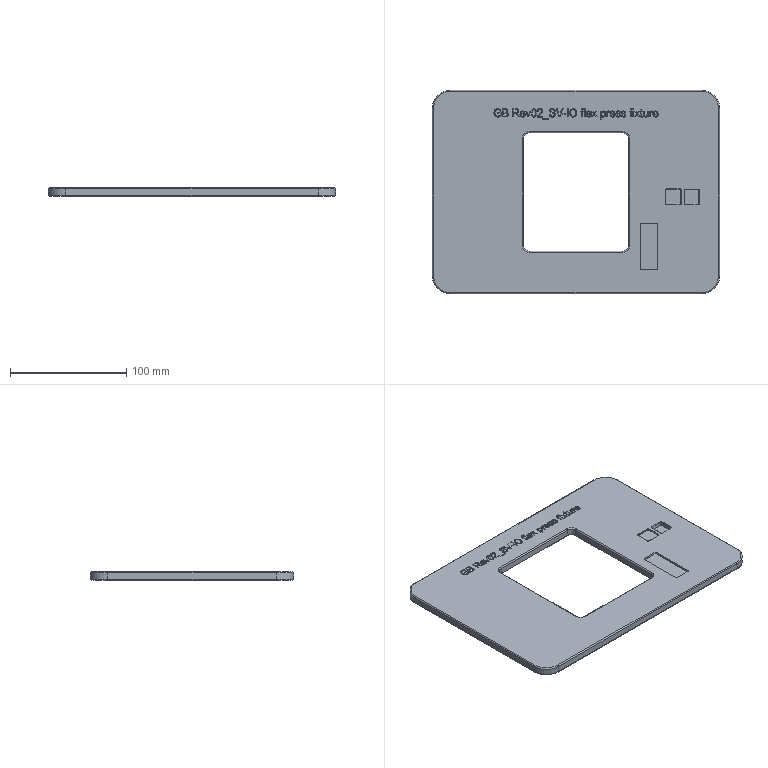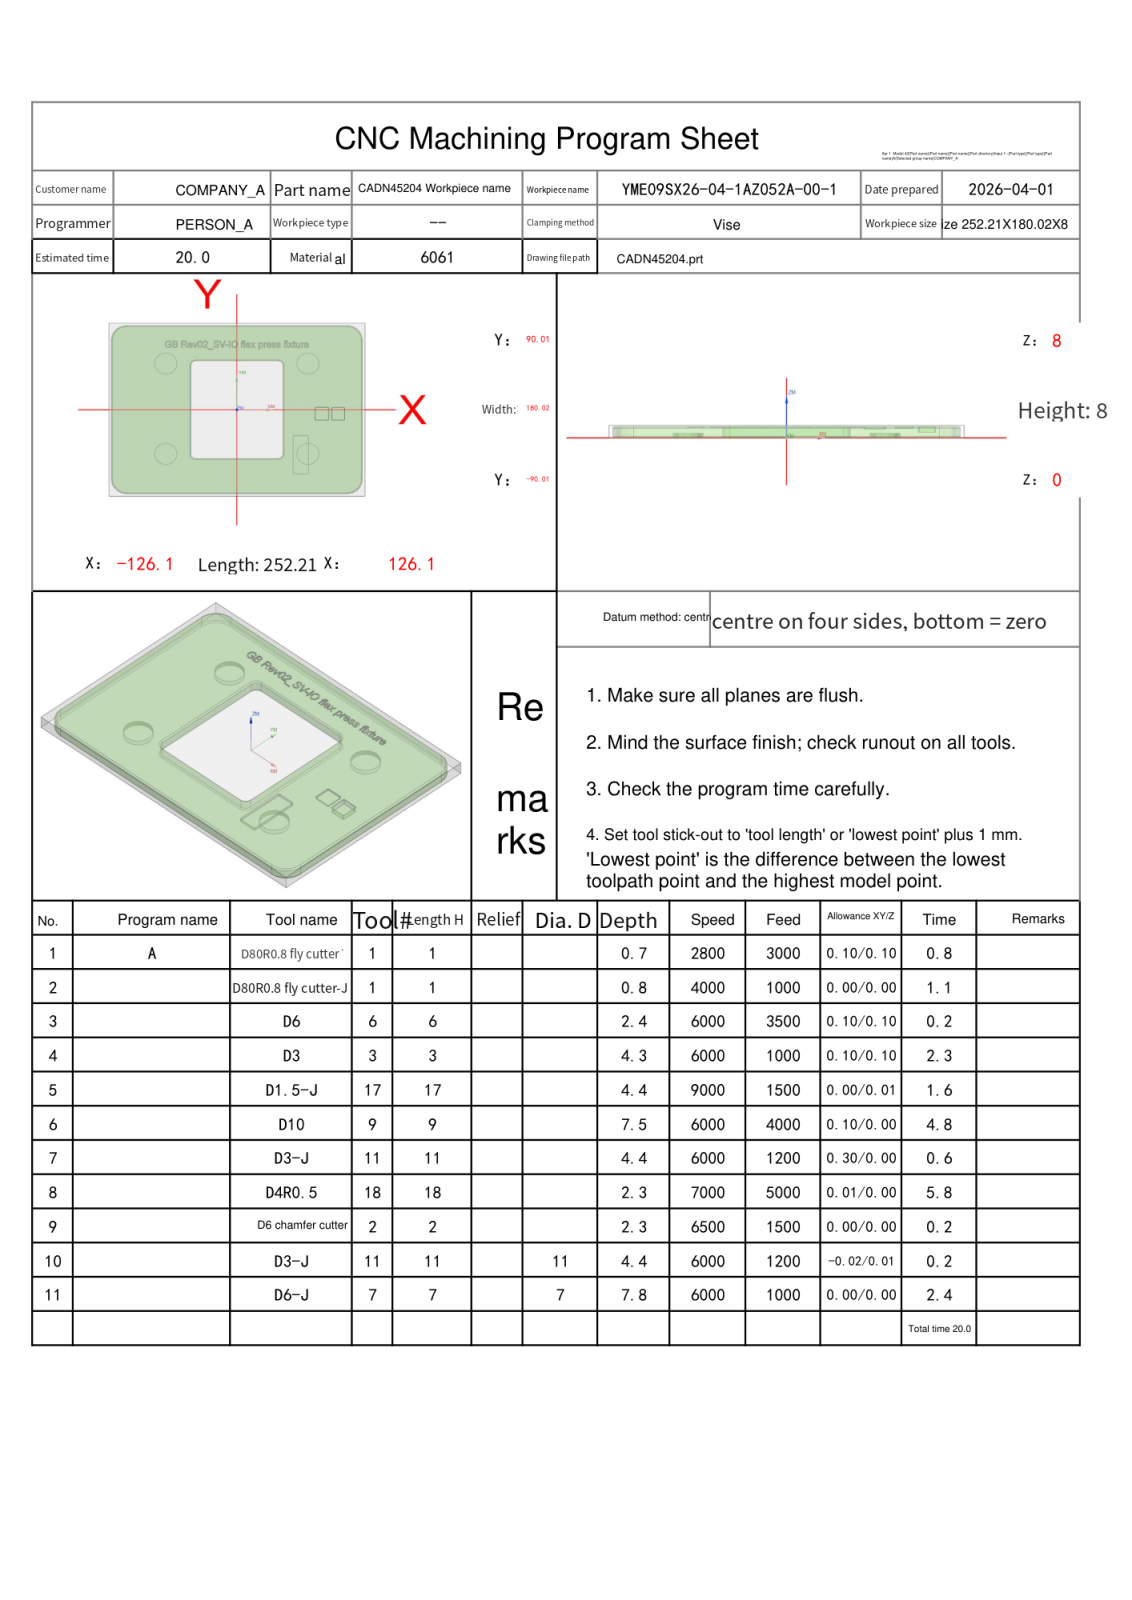NC program | NX | posted by the shop | part box 247.208 x 175.016 x 7.2 mm
Lines 7290 to 7606 of 29502:
N6 T09 M06
(D10  D=10. R=0. H=09 ce=0.10 di=0.00)
G00 G90 G54 X0.0 Y-92.608 M03 S6000
G43 H09 Z27.2
M08
Z7.7
G01 X-108.604 Z7.639 F4000.
G02 X-128.704 Y-72.508 Z7.621 I0.0 J20.1
G01 Y72.508 Z7.539
G02 X-108.604 Y92.608 Z7.521 I20.1 J0.0
G01 X108.604 Z7.399
G02 X128.704 Y72.508 Z7.381 I0.0 J-20.1
G01 Y-72.508 Z7.299
G02 X108.604 Y-92.608 Z7.281 I-20.1 J0.0
G01 X-108.604 Z7.159
G02 X-128.704 Y-72.508 Z7.141 I0.0 J20.1
G01 Y72.508 Z7.059
G02 X-108.604 Y92.608 Z7.041 I20.1 J0.0
G01 X108.604 Z6.919
G02 X128.704 Y72.508 Z6.901 I0.0 J-20.1
G01 Y-72.508 Z6.819
G02 X108.604 Y-92.608 Z6.801 I-20.1 J0.0
G01 X-108.604 Z6.679
G02 X-128.704 Y-72.508 Z6.661 I0.0 J20.1
G01 Y72.508 Z6.579
G02 X-108.604 Y92.608 Z6.561 I20.1 J0.0
G01 X108.604 Z6.439
G02 X128.704 Y72.508 Z6.421 I0.0 J-20.1
G01 Y-72.508 Z6.339
G02 X108.604 Y-92.608 Z6.321 I-20.1 J0.0
G01 X-108.604 Z6.199
G02 X-128.704 Y-72.508 Z6.181 I0.0 J20.1
G01 Y72.508 Z6.099
G02 X-108.604 Y92.608 Z6.081 I20.1 J0.0
G01 X108.604 Z5.959
G02 X128.704 Y72.508 Z5.941 I0.0 J-20.1
G01 Y-72.508 Z5.859
G02 X108.604 Y-92.608 Z5.841 I-20.1 J0.0
G01 X-108.604 Z5.719
G02 X-128.704 Y-72.508 Z5.701 I0.0 J20.1
G01 Y72.508 Z5.619
G02 X-108.604 Y92.608 Z5.601 I20.1 J0.0
G01 X108.604 Z5.479
G02 X128.704 Y72.508 Z5.461 I0.0 J-20.1
G01 Y-72.508 Z5.379
G02 X108.604 Y-92.608 Z5.361 I-20.1 J0.0
G01 X-108.604 Z5.239
G02 X-128.704 Y-72.508 Z5.221 I0.0 J20.1
G01 Y72.508 Z5.139
G02 X-108.604 Y92.608 Z5.121 I20.1 J0.0
G01 X108.604 Z4.999
G02 X128.704 Y72.508 Z4.981 I0.0 J-20.1
G01 Y-72.508 Z4.899
G02 X108.604 Y-92.608 Z4.881 I-20.1 J0.0
G01 X-108.604 Z4.759
G02 X-128.704 Y-72.508 Z4.741 I0.0 J20.1
G01 Y72.508 Z4.659
G02 X-108.604 Y92.608 Z4.641 I20.1 J0.0
G01 X108.604 Z4.519
G02 X128.704 Y72.508 Z4.501 I0.0 J-20.1
G01 Y-72.508 Z4.419
G02 X108.604 Y-92.608 Z4.401 I-20.1 J0.0
G01 X-108.604 Z4.279
G02 X-128.704 Y-72.508 Z4.261 I0.0 J20.1
G01 Y72.508 Z4.179
G02 X-108.604 Y92.608 Z4.161 I20.1 J0.0
G01 X108.604 Z4.039
G02 X128.704 Y72.508 Z4.021 I0.0 J-20.1
G01 Y-72.508 Z3.939
G02 X108.604 Y-92.608 Z3.921 I-20.1 J0.0
G01 X-108.604 Z3.799
G02 X-128.704 Y-72.508 Z3.781 I0.0 J20.1
G01 Y72.508 Z3.699
G02 X-108.604 Y92.608 Z3.681 I20.1 J0.0
G01 X108.604 Z3.559
G02 X128.704 Y72.508 Z3.541 I0.0 J-20.1
G01 Y-72.508 Z3.459
G02 X108.604 Y-92.608 Z3.441 I-20.1 J0.0
G01 X-108.604 Z3.319
G02 X-128.704 Y-72.508 Z3.301 I0.0 J20.1
G01 Y72.508 Z3.219
G02 X-108.604 Y92.608 Z3.201 I20.1 J0.0
G01 X108.604 Z3.079
G02 X128.704 Y72.508 Z3.061 I0.0 J-20.1
G01 Y-72.508 Z2.979
G02 X108.604 Y-92.608 Z2.961 I-20.1 J0.0
G01 X-108.604 Z2.839
G02 X-128.704 Y-72.508 Z2.821 I0.0 J20.1
G01 Y72.508 Z2.739
G02 X-108.604 Y92.608 Z2.721 I20.1 J0.0
G01 X108.604 Z2.599
G02 X128.704 Y72.508 Z2.581 I0.0 J-20.1
G01 Y-72.508 Z2.499
G02 X108.604 Y-92.608 Z2.481 I-20.1 J0.0
G01 X-108.604 Z2.359
G02 X-128.704 Y-72.508 Z2.341 I0.0 J20.1
G01 Y72.508 Z2.259
G02 X-108.604 Y92.608 Z2.241 I20.1 J0.0
G01 X108.604 Z2.119
G02 X128.704 Y72.508 Z2.101 I0.0 J-20.1
G01 Y-72.508 Z2.019
G02 X108.604 Y-92.608 Z2.001 I-20.1 J0.0
G01 X-108.604 Z1.879
G02 X-128.704 Y-72.508 Z1.861 I0.0 J20.1
G01 Y72.508 Z1.779
G02 X-108.604 Y92.608 Z1.761 I20.1 J0.0
G01 X108.604 Z1.639
G02 X128.704 Y72.508 Z1.621 I0.0 J-20.1
G01 Y-72.508 Z1.539
G02 X108.604 Y-92.608 Z1.521 I-20.1 J0.0
G01 X-108.604 Z1.399
G02 X-128.704 Y-72.508 Z1.381 I0.0 J20.1
G01 Y72.508 Z1.299
G02 X-108.604 Y92.608 Z1.281 I20.1 J0.0
G01 X108.604 Z1.159
G02 X128.704 Y72.508 Z1.141 I0.0 J-20.1
G01 Y-72.508 Z1.059
G02 X108.604 Y-92.608 Z1.041 I-20.1 J0.0
G01 X-108.604 Z.919
G02 X-128.704 Y-72.508 Z.901 I0.0 J20.1
G01 Y72.508 Z.819
G02 X-108.604 Y92.608 Z.801 I20.1 J0.0
G01 X108.604 Z.679
G02 X128.704 Y72.508 Z.661 I0.0 J-20.1
G01 Y-72.508 Z.579
G02 X108.604 Y-92.608 Z.561 I-20.1 J0.0
G01 X0.0 Z.5
X-108.604
G02 X-128.704 Y-72.508 I0.0 J20.1
G01 Y72.508
G02 X-108.604 Y92.608 I20.1 J0.0
G01 X108.604
G02 X128.704 Y72.508 I0.0 J-20.1
G01 Y-72.508
G02 X108.604 Y-92.608 I-20.1 J0.0
G01 X0.0
X-.5
Z1.5
G00 Z27.2
X40.263 Y0.0
Z7.7
G01 Y45.746 Z7.636
X-40.259 Z7.524
Y-45.746 Z7.396
X40.263 Z7.284
Y45.746 Z7.156
X-40.259 Z7.044
Y-45.746 Z6.916
X40.263 Z6.804
Y45.746 Z6.676
X-40.259 Z6.564
Y-45.746 Z6.436
X40.263 Z6.324
Y45.746 Z6.196
X-40.259 Z6.084
Y-45.746 Z5.956
X40.263 Z5.844
Y45.746 Z5.716
X-40.259 Z5.604
Y-45.746 Z5.476
X40.263 Z5.364
Y45.746 Z5.236
X-40.259 Z5.124
Y-45.746 Z4.996
X40.263 Z4.884
Y45.746 Z4.756
X-40.259 Z4.644
Y-45.746 Z4.516
X40.263 Z4.404
Y45.746 Z4.276
X-40.259 Z4.164
Y-45.746 Z4.036
X40.263 Z3.924
Y45.746 Z3.796
X-40.259 Z3.684
Y-45.746 Z3.556
X40.263 Z3.444
Y45.746 Z3.316
X-40.259 Z3.204
Y-45.746 Z3.076
X40.263 Z2.964
Y45.746 Z2.836
X-40.259 Z2.724
Y-45.746 Z2.596
X40.263 Z2.484
Y45.746 Z2.356
X-40.259 Z2.244
Y-45.746 Z2.116
X40.263 Z2.004
Y45.746 Z1.876
X-40.259 Z1.764
Y-45.746 Z1.636
X40.263 Z1.524
Y45.746 Z1.396
X-40.259 Z1.284
Y-45.746 Z1.156
X40.263 Z1.044
Y45.746 Z.916
X-40.259 Z.804
Y-45.746 Z.676
X40.263 Z.564
Y0.0 Z.5
Y45.746
X-40.259
Y-45.746
X40.263
Y0.0
Y.5
Z1.5
G00 Z27.2
G91 G28 Z0.0
M05
M09
G91 G28 Z0.0
M01
N7 T11 M06
(D3-J  D=3. R=0. H=11 ce=0.30 di=0.00)
G00 G90 G54 X57.262 Y-41.973 M03 S6000
G43 H11 Z27.2
M08
Z7.
G01 Y-28.619 Z6.534 F1200.
X68.662 Z6.136
Y-46.819 Z5.5
Y-65.019
X57.262
Y-28.619
X68.662
Y-46.819
X66.562
Y-62.919
X59.362
Y-30.719
X66.562
Y-46.819
X64.462
Y-60.819
X61.462
Y-32.819
X64.462
Y-46.819
X63.112
Y-59.469
X62.812
Y-34.169
X63.112
Y-46.819
Y-47.319
X64.912
Z6.
G00 Z27.2
G00 G90 X87.958 Y.485 M03 S6000
Z27.2
Z7.58
G01 X88.485 Z7.562 F800.
Y-8.934 Z7.233
X79.044 Z6.903
Y.485 Z6.574
X88.485 Z6.244
Y-4.225 Z6.08
Y-8.934
X79.044
Y.485
X88.485
Y-4.225
X86.385
Y-6.834
X81.144
Y-1.615
X86.385
Y-4.225
X84.285
Y-4.734
X83.244
Y-3.715
X84.285
Y-4.225
Y-4.725
X86.085
Z6.58
G00 Z27.2
G00 G90 X101.221 Y.266 M03 S6000
Z27.2
Z5.058
G01 X104.052 Z4.96 F800.
Y-8.934 Z4.638
X95.49 Z4.339
Y.266 Z4.018
X104.052 Z3.719
Y-4.334 Z3.558
Y-8.934
X95.49
Y.266
X104.052
Y-4.334
X101.952
Y-6.834
X97.59
Y-1.834
X101.952
Y-4.334
X99.852
Y-4.734
X99.69
Y-3.934
X99.852
Y-4.334
Y-4.734
X99.752
Y-6.534
Z4.058
G00 Z27.2
G91 G28 Z0.0
M05
M09
G91 G28 Z0.0
M01